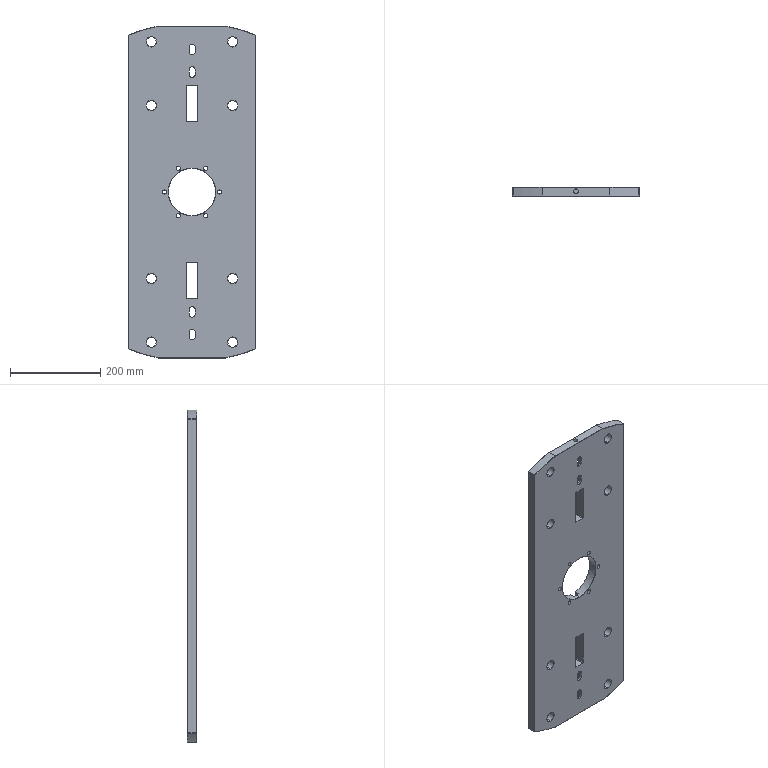Part | SolidWorks | features Cut 5, HoleWzd 4, MirrorPattern 4, Fillet 2, ICE 2, Chamfer 1, Extrusion 1 | 1 solid | 174 faces | box 280 x 20 x 735 mm | volume 3611529 mm3 | cylinder 70 | plane 60 | cone 44 | commonest cylinder face diameters 22 x16 3 x12 9 x12 13.5 x12 4 x8 10.2 x4